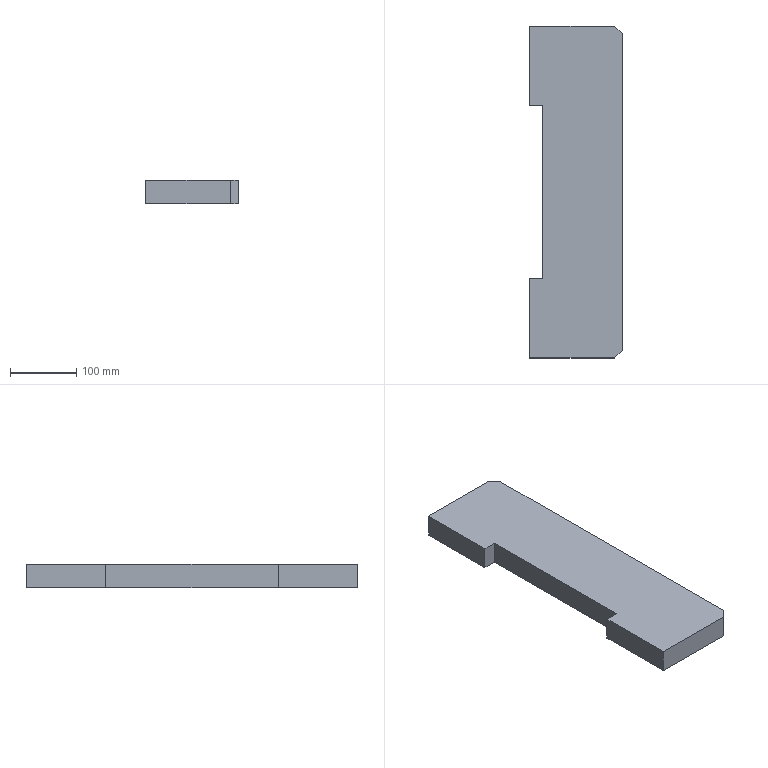Part | SolidWorks | features Chamfer 1, Extrusion 1 | 1 solid | 12 faces | box 140 x 500 x 35 mm | volume 2262960 mm3 | plane 12
STEP:
#1=CARTESIAN_POINT('',(0.,-488.,35.));
#2=VERTEX_POINT('',#1);
#3=CARTESIAN_POINT('',(0.,-12.,35.));
#4=VERTEX_POINT('',#3);
#5=CARTESIAN_POINT('',(0.,0.,35.));
#6=DIRECTION('',(0.,1.,0.));
#7=VECTOR('',#6,1000.);
#8=LINE('',#5,#7);
#9=EDGE_CURVE('',#2,#4,#8,.T.);
#10=ORIENTED_EDGE('',*,*,#9,.F.);
#11=CARTESIAN_POINT('',(0.,-488.,0.));
#12=VERTEX_POINT('',#11);
#13=CARTESIAN_POINT('',(0.,-488.,35.));
#14=DIRECTION('',(0.,0.,-1.));
#15=VECTOR('',#14,1000.);
#16=LINE('',#13,#15);
#17=EDGE_CURVE('',#2,#12,#16,.T.);
#18=ORIENTED_EDGE('',*,*,#17,.T.);
#19=CARTESIAN_POINT('',(0.,-12.,0.));
#20=VERTEX_POINT('',#19);
#21=CARTESIAN_POINT('',(0.,0.,0.));
#22=DIRECTION('',(0.,1.,0.));
#23=VECTOR('',#22,1000.);
#24=LINE('',#21,#23);
#25=EDGE_CURVE('',#12,#20,#24,.T.);
#26=ORIENTED_EDGE('',*,*,#25,.T.);
#27=CARTESIAN_POINT('',(0.,-12.,35.));
#28=DIRECTION('',(0.,0.,1.));
#29=VECTOR('',#28,1000.);
#30=LINE('',#27,#29);
#31=EDGE_CURVE('',#20,#4,#30,.T.);
#32=ORIENTED_EDGE('',*,*,#31,.T.);
#33=EDGE_LOOP('',(#10,#18,#26,#32));
#34=FACE_OUTER_BOUND('',#33,.T.);
#35=CARTESIAN_POINT('',(0.,0.,35.));
#36=DIRECTION('',(-1.,0.,0.));
#37=DIRECTION('',(0.,-1.,0.));
#38=AXIS2_PLACEMENT_3D('',#35,#36,#37);
#39=PLANE('',#38);
#40=ADVANCED_FACE('',(#34),#39,.F.);
#41=CARTESIAN_POINT('',(-12.,0.,35.));
#42=VERTEX_POINT('',#41);
#43=CARTESIAN_POINT('',(-140.,0.,35.));
#44=VERTEX_POINT('',#43);
#45=CARTESIAN_POINT('',(-140.,0.,35.));
#46=DIRECTION('',(-1.,0.,0.));
#47=VECTOR('',#46,1000.);
#48=LINE('',#45,#47);
#49=EDGE_CURVE('',#42,#44,#48,.T.);
#50=ORIENTED_EDGE('',*,*,#49,.F.);
#51=CARTESIAN_POINT('',(-12.,0.,0.));
#52=VERTEX_POINT('',#51);
#53=CARTESIAN_POINT('',(-12.,0.,35.));
#54=DIRECTION('',(0.,0.,-1.));
#55=VECTOR('',#54,1000.);
#56=LINE('',#53,#55);
#57=EDGE_CURVE('',#42,#52,#56,.T.);
#58=ORIENTED_EDGE('',*,*,#57,.T.);
#59=CARTESIAN_POINT('',(-140.,0.,0.));
#60=VERTEX_POINT('',#59);
#61=CARTESIAN_POINT('',(-140.,0.,0.));
#62=DIRECTION('',(-1.,0.,0.));
#63=VECTOR('',#62,1000.);
#64=LINE('',#61,#63);
#65=EDGE_CURVE('',#52,#60,#64,.T.);
#66=ORIENTED_EDGE('',*,*,#65,.T.);
#67=CARTESIAN_POINT('',(-140.,0.,35.));
#68=DIRECTION('',(0.,0.,-1.));
#69=VECTOR('',#68,1000.);
#70=LINE('',#67,#69);
#71=EDGE_CURVE('',#44,#60,#70,.T.);
#72=ORIENTED_EDGE('',*,*,#71,.F.);
#73=EDGE_LOOP('',(#50,#58,#66,#72));
#74=FACE_OUTER_BOUND('',#73,.T.);
#75=CARTESIAN_POINT('',(-140.,0.,35.));
#76=DIRECTION('',(0.,-1.,0.));
#77=DIRECTION('',(0.,0.,-1.));
#78=AXIS2_PLACEMENT_3D('',#75,#76,#77);
#79=PLANE('',#78);
#80=ADVANCED_FACE('',(#74),#79,.F.);
#81=CARTESIAN_POINT('',(-140.,-120.,0.));
#82=VERTEX_POINT('',#81);
#83=CARTESIAN_POINT('',(-140.,0.,0.));
#84=DIRECTION('',(0.,-1.,0.));
#85=VECTOR('',#84,1000.);
#86=LINE('',#83,#85);
#87=EDGE_CURVE('',#60,#82,#86,.T.);
#88=ORIENTED_EDGE('',*,*,#87,.T.);
#89=CARTESIAN_POINT('',(-140.,-120.,35.));
#90=VERTEX_POINT('',#89);
#91=CARTESIAN_POINT('',(-140.,-120.,35.));
#92=DIRECTION('',(0.,0.,-1.));
#93=VECTOR('',#92,1000.);
#94=LINE('',#91,#93);
#95=EDGE_CURVE('',#90,#82,#94,.T.);
#96=ORIENTED_EDGE('',*,*,#95,.F.);
#97=CARTESIAN_POINT('',(-140.,0.,35.));
#98=DIRECTION('',(0.,-1.,0.));
#99=VECTOR('',#98,1000.);
#100=LINE('',#97,#99);
#101=EDGE_CURVE('',#44,#90,#100,.T.);
#102=ORIENTED_EDGE('',*,*,#101,.F.);
#103=ORIENTED_EDGE('',*,*,#71,.T.);
#104=EDGE_LOOP('',(#88,#96,#102,#103));
#105=FACE_OUTER_BOUND('',#104,.T.);
#106=CARTESIAN_POINT('',(-140.,0.,35.));
#107=DIRECTION('',(1.,0.,0.));
#108=DIRECTION('',(0.,1.,0.));
#109=AXIS2_PLACEMENT_3D('',#106,#107,#108);
#110=PLANE('',#109);
#111=ADVANCED_FACE('',(#105),#110,.F.);
#112=CARTESIAN_POINT('',(-120.,-120.,0.));
#113=VERTEX_POINT('',#112);
#114=CARTESIAN_POINT('',(-120.,-120.,0.));
#115=DIRECTION('',(1.,0.,0.));
#116=VECTOR('',#115,1000.);
#117=LINE('',#114,#116);
#118=EDGE_CURVE('',#82,#113,#117,.T.);
#119=ORIENTED_EDGE('',*,*,#118,.T.);
#120=CARTESIAN_POINT('',(-120.,-120.,35.));
#121=VERTEX_POINT('',#120);
#122=CARTESIAN_POINT('',(-120.,-120.,35.));
#123=DIRECTION('',(0.,0.,-1.));
#124=VECTOR('',#123,1000.);
#125=LINE('',#122,#124);
#126=EDGE_CURVE('',#121,#113,#125,.T.);
#127=ORIENTED_EDGE('',*,*,#126,.F.);
#128=CARTESIAN_POINT('',(-120.,-120.,35.));
#129=DIRECTION('',(1.,0.,0.));
#130=VECTOR('',#129,1000.);
#131=LINE('',#128,#130);
#132=EDGE_CURVE('',#90,#121,#131,.T.);
#133=ORIENTED_EDGE('',*,*,#132,.F.);
#134=ORIENTED_EDGE('',*,*,#95,.T.);
#135=EDGE_LOOP('',(#119,#127,#133,#134));
#136=FACE_OUTER_BOUND('',#135,.T.);
#137=CARTESIAN_POINT('',(-120.,-120.,35.));
#138=DIRECTION('',(0.,1.,0.));
#139=DIRECTION('',(0.,0.,1.));
#140=AXIS2_PLACEMENT_3D('',#137,#138,#139);
#141=PLANE('',#140);
#142=ADVANCED_FACE('',(#136),#141,.F.);
#143=CARTESIAN_POINT('',(-120.,-380.,0.));
#144=VERTEX_POINT('',#143);
#145=CARTESIAN_POINT('',(-120.,-120.,0.));
#146=DIRECTION('',(0.,-1.,0.));
#147=VECTOR('',#146,1000.);
#148=LINE('',#145,#147);
#149=EDGE_CURVE('',#113,#144,#148,.T.);
#150=ORIENTED_EDGE('',*,*,#149,.T.);
#151=CARTESIAN_POINT('',(-120.,-380.,35.));
#152=VERTEX_POINT('',#151);
#153=CARTESIAN_POINT('',(-120.,-380.,35.));
#154=DIRECTION('',(0.,0.,-1.));
#155=VECTOR('',#154,1000.);
#156=LINE('',#153,#155);
#157=EDGE_CURVE('',#152,#144,#156,.T.);
#158=ORIENTED_EDGE('',*,*,#157,.F.);
#159=CARTESIAN_POINT('',(-120.,-120.,35.));
#160=DIRECTION('',(0.,-1.,0.));
#161=VECTOR('',#160,1000.);
#162=LINE('',#159,#161);
#163=EDGE_CURVE('',#121,#152,#162,.T.);
#164=ORIENTED_EDGE('',*,*,#163,.F.);
#165=ORIENTED_EDGE('',*,*,#126,.T.);
#166=EDGE_LOOP('',(#150,#158,#164,#165));
#167=FACE_OUTER_BOUND('',#166,.T.);
#168=CARTESIAN_POINT('',(-120.,-120.,35.));
#169=DIRECTION('',(1.,0.,0.));
#170=DIRECTION('',(0.,1.,0.));
#171=AXIS2_PLACEMENT_3D('',#168,#169,#170);
#172=PLANE('',#171);
#173=ADVANCED_FACE('',(#167),#172,.F.);
#174=CARTESIAN_POINT('',(-140.,-380.,0.));
#175=VERTEX_POINT('',#174);
#176=CARTESIAN_POINT('',(-120.,-380.,0.));
#177=DIRECTION('',(-1.,0.,0.));
#178=VECTOR('',#177,1000.);
#179=LINE('',#176,#178);
#180=EDGE_CURVE('',#144,#175,#179,.T.);
#181=ORIENTED_EDGE('',*,*,#180,.T.);
#182=CARTESIAN_POINT('',(-140.,-380.,35.));
#183=VERTEX_POINT('',#182);
#184=CARTESIAN_POINT('',(-140.,-380.,35.));
#185=DIRECTION('',(0.,0.,-1.));
#186=VECTOR('',#185,1000.);
#187=LINE('',#184,#186);
#188=EDGE_CURVE('',#183,#175,#187,.T.);
#189=ORIENTED_EDGE('',*,*,#188,.F.);
#190=CARTESIAN_POINT('',(-120.,-380.,35.));
#191=DIRECTION('',(-1.,0.,0.));
#192=VECTOR('',#191,1000.);
#193=LINE('',#190,#192);
#194=EDGE_CURVE('',#152,#183,#193,.T.);
#195=ORIENTED_EDGE('',*,*,#194,.F.);
#196=ORIENTED_EDGE('',*,*,#157,.T.);
#197=EDGE_LOOP('',(#181,#189,#195,#196));
#198=FACE_OUTER_BOUND('',#197,.T.);
#199=CARTESIAN_POINT('',(-120.,-380.,35.));
#200=DIRECTION('',(0.,-1.,0.));
#201=DIRECTION('',(0.,0.,-1.));
#202=AXIS2_PLACEMENT_3D('',#199,#200,#201);
#203=PLANE('',#202);
#204=ADVANCED_FACE('',(#198),#203,.F.);
#205=CARTESIAN_POINT('',(-140.,-500.,0.));
#206=VERTEX_POINT('',#205);
#207=CARTESIAN_POINT('',(-140.,-500.,0.));
#208=DIRECTION('',(0.,-1.,0.));
#209=VECTOR('',#208,1000.);
#210=LINE('',#207,#209);
#211=EDGE_CURVE('',#175,#206,#210,.T.);
#212=ORIENTED_EDGE('',*,*,#211,.T.);
#213=CARTESIAN_POINT('',(-140.,-500.,35.));
#214=VERTEX_POINT('',#213);
#215=CARTESIAN_POINT('',(-140.,-500.,35.));
#216=DIRECTION('',(0.,0.,-1.));
#217=VECTOR('',#216,1000.);
#218=LINE('',#215,#217);
#219=EDGE_CURVE('',#214,#206,#218,.T.);
#220=ORIENTED_EDGE('',*,*,#219,.F.);
#221=CARTESIAN_POINT('',(-140.,-500.,35.));
#222=DIRECTION('',(0.,-1.,0.));
#223=VECTOR('',#222,1000.);
#224=LINE('',#221,#223);
#225=EDGE_CURVE('',#183,#214,#224,.T.);
#226=ORIENTED_EDGE('',*,*,#225,.F.);
#227=ORIENTED_EDGE('',*,*,#188,.T.);
#228=EDGE_LOOP('',(#212,#220,#226,#227));
#229=FACE_OUTER_BOUND('',#228,.T.);
#230=CARTESIAN_POINT('',(-140.,-500.,35.));
#231=DIRECTION('',(1.,0.,0.));
#232=DIRECTION('',(0.,0.,-1.));
#233=AXIS2_PLACEMENT_3D('',#230,#231,#232);
#234=PLANE('',#233);
#235=ADVANCED_FACE('',(#229),#234,.F.);
#236=CARTESIAN_POINT('',(-12.,-500.,0.));
#237=VERTEX_POINT('',#236);
#238=CARTESIAN_POINT('',(0.,-500.,0.));
#239=DIRECTION('',(1.,0.,0.));
#240=VECTOR('',#239,1000.);
#241=LINE('',#238,#240);
#242=EDGE_CURVE('',#206,#237,#241,.T.);
#243=ORIENTED_EDGE('',*,*,#242,.T.);
#244=CARTESIAN_POINT('',(-12.,-500.,35.));
#245=VERTEX_POINT('',#244);
#246=CARTESIAN_POINT('',(-12.,-500.,35.));
#247=DIRECTION('',(0.,0.,1.));
#248=VECTOR('',#247,1000.);
#249=LINE('',#246,#248);
#250=EDGE_CURVE('',#237,#245,#249,.T.);
#251=ORIENTED_EDGE('',*,*,#250,.T.);
#252=CARTESIAN_POINT('',(0.,-500.,35.));
#253=DIRECTION('',(1.,0.,0.));
#254=VECTOR('',#253,1000.);
#255=LINE('',#252,#254);
#256=EDGE_CURVE('',#214,#245,#255,.T.);
#257=ORIENTED_EDGE('',*,*,#256,.F.);
#258=ORIENTED_EDGE('',*,*,#219,.T.);
#259=EDGE_LOOP('',(#243,#251,#257,#258));
#260=FACE_OUTER_BOUND('',#259,.T.);
#261=CARTESIAN_POINT('',(0.,-500.,35.));
#262=DIRECTION('',(0.,1.,0.));
#263=DIRECTION('',(0.,0.,1.));
#264=AXIS2_PLACEMENT_3D('',#261,#262,#263);
#265=PLANE('',#264);
#266=ADVANCED_FACE('',(#260),#265,.F.);
#267=ORIENTED_EDGE('',*,*,#256,.T.);
#268=CARTESIAN_POINT('',(0.,-488.,35.));
#269=DIRECTION('',(0.7071,0.7071,0.));
#270=VECTOR('',#269,1000.);
#271=LINE('',#268,#270);
#272=EDGE_CURVE('',#245,#2,#271,.T.);
#273=ORIENTED_EDGE('',*,*,#272,.T.);
#274=ORIENTED_EDGE('',*,*,#9,.T.);
#275=CARTESIAN_POINT('',(-12.,0.,35.));
#276=DIRECTION('',(-0.7071,0.7071,0.));
#277=VECTOR('',#276,1000.);
#278=LINE('',#275,#277);
#279=EDGE_CURVE('',#4,#42,#278,.T.);
#280=ORIENTED_EDGE('',*,*,#279,.T.);
#281=ORIENTED_EDGE('',*,*,#49,.T.);
#282=ORIENTED_EDGE('',*,*,#101,.T.);
#283=ORIENTED_EDGE('',*,*,#132,.T.);
#284=ORIENTED_EDGE('',*,*,#163,.T.);
#285=ORIENTED_EDGE('',*,*,#194,.T.);
#286=ORIENTED_EDGE('',*,*,#225,.T.);
#287=EDGE_LOOP('',(#267,#273,#274,#280,#281,#282,#283,#284,#285,#286));
#288=FACE_OUTER_BOUND('',#287,.T.);
#289=CARTESIAN_POINT('',(0.,0.,35.));
#290=DIRECTION('',(0.,0.,-1.));
#291=DIRECTION('',(-1.,0.,0.));
#292=AXIS2_PLACEMENT_3D('',#289,#290,#291);
#293=PLANE('',#292);
#294=ADVANCED_FACE('',(#288),#293,.F.);
#295=ORIENTED_EDGE('',*,*,#25,.F.);
#296=CARTESIAN_POINT('',(244.,-244.,0.));
#297=DIRECTION('',(-0.7071,-0.7071,0.));
#298=VECTOR('',#297,1000.);
#299=LINE('',#296,#298);
#300=EDGE_CURVE('',#12,#237,#299,.T.);
#301=ORIENTED_EDGE('',*,*,#300,.T.);
#302=ORIENTED_EDGE('',*,*,#242,.F.);
#303=ORIENTED_EDGE('',*,*,#211,.F.);
#304=ORIENTED_EDGE('',*,*,#180,.F.);
#305=ORIENTED_EDGE('',*,*,#149,.F.);
#306=ORIENTED_EDGE('',*,*,#118,.F.);
#307=ORIENTED_EDGE('',*,*,#87,.F.);
#308=ORIENTED_EDGE('',*,*,#65,.F.);
#309=CARTESIAN_POINT('',(-6.,-6.,0.));
#310=DIRECTION('',(0.7071,-0.7071,0.));
#311=VECTOR('',#310,1000.);
#312=LINE('',#309,#311);
#313=EDGE_CURVE('',#52,#20,#312,.T.);
#314=ORIENTED_EDGE('',*,*,#313,.T.);
#315=EDGE_LOOP('',(#295,#301,#302,#303,#304,#305,#306,#307,#308,#314));
#316=FACE_OUTER_BOUND('',#315,.T.);
#317=CARTESIAN_POINT('',(0.,0.,0.));
#318=DIRECTION('',(0.,0.,-1.));
#319=DIRECTION('',(-1.,0.,0.));
#320=AXIS2_PLACEMENT_3D('',#317,#318,#319);
#321=PLANE('',#320);
#322=ADVANCED_FACE('',(#316),#321,.T.);
#323=ORIENTED_EDGE('',*,*,#272,.F.);
#324=ORIENTED_EDGE('',*,*,#250,.F.);
#325=ORIENTED_EDGE('',*,*,#300,.F.);
#326=ORIENTED_EDGE('',*,*,#17,.F.);
#327=EDGE_LOOP('',(#323,#324,#325,#326));
#328=FACE_OUTER_BOUND('',#327,.T.);
#329=CARTESIAN_POINT('',(0.,-488.,35.));
#330=DIRECTION('',(-0.7071,0.7071,0.));
#331=DIRECTION('',(0.,0.,-1.));
#332=AXIS2_PLACEMENT_3D('',#329,#330,#331);
#333=PLANE('',#332);
#334=ADVANCED_FACE('',(#328),#333,.F.);
#335=ORIENTED_EDGE('',*,*,#279,.F.);
#336=ORIENTED_EDGE('',*,*,#31,.F.);
#337=ORIENTED_EDGE('',*,*,#313,.F.);
#338=ORIENTED_EDGE('',*,*,#57,.F.);
#339=EDGE_LOOP('',(#335,#336,#337,#338));
#340=FACE_OUTER_BOUND('',#339,.T.);
#341=CARTESIAN_POINT('',(-12.,0.,35.));
#342=DIRECTION('',(-0.7071,-0.7071,0.));
#343=DIRECTION('',(0.,0.,-1.));
#344=AXIS2_PLACEMENT_3D('',#341,#342,#343);
#345=PLANE('',#344);
#346=ADVANCED_FACE('',(#340),#345,.F.);
#347=CLOSED_SHELL('',(#40,#80,#111,#142,#173,#204,#235,#266,#294,#322,#334,#346));
#348=MANIFOLD_SOLID_BREP('',#347);
#349=CARTESIAN_POINT('',(0.,0.,0.));
#350=DIRECTION('',(0.,0.,1.));
#351=DIRECTION('',(1.,0.,0.));
#352=AXIS2_PLACEMENT_3D('',#349,#350,#351);
#353=(LENGTH_UNIT()NAMED_UNIT(*)SI_UNIT(.MILLI.,.METRE.));
#354=UNCERTAINTY_MEASURE_WITH_UNIT(LENGTH_MEASURE(0.00001),#353,'','');
#355=(NAMED_UNIT(*)PLANE_ANGLE_UNIT()SI_UNIT($,.RADIAN.));
#356=(NAMED_UNIT(*)SI_UNIT($,.STERADIAN.)SOLID_ANGLE_UNIT());
#357=(GEOMETRIC_REPRESENTATION_CONTEXT(3)GLOBAL_UNCERTAINTY_ASSIGNED_CONTEXT((#354))GLOBAL_UNIT_ASSIGNED_CONTEXT((#353,#355,#356))REPRESENTATION_CONTEXT('',''));
#358=ADVANCED_BREP_SHAPE_REPRESENTATION('',(#348,#352),#357);